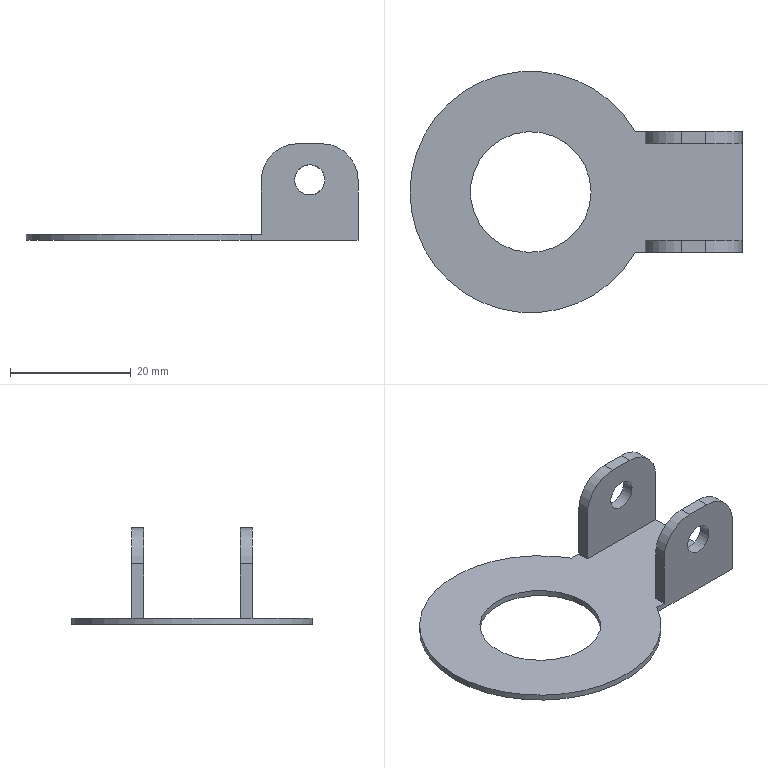Part | NX | features DATUM_CSYS 5, EXTRUDE 4, SKETCH 4, BLEND 1 | 1 solid | 19 faces | box 55 x 40 x 16 mm | volume 2079 mm3 | plane 11 | cylinder 8 | commonest cylinder face diameters 12 x4 5 x2 20 x1 40 x1
STEP:
#1=CARTESIAN_POINT('',(17.321,10.,0.));
#2=VERTEX_POINT('',#1);
#3=CARTESIAN_POINT('',(17.321,-10.,0.));
#4=VERTEX_POINT('',#3);
#5=CARTESIAN_POINT('',(0.,0.,0.));
#6=DIRECTION('',(0.,0.,1.));
#7=DIRECTION('',(1.,0.,0.));
#8=AXIS2_PLACEMENT_3D('',#5,#6,#7);
#9=CIRCLE('',#8,20.);
#10=EDGE_CURVE('',#2,#4,#9,.T.);
#11=ORIENTED_EDGE('',*,*,#10,.T.);
#12=CARTESIAN_POINT('',(17.321,-10.,1.));
#13=VERTEX_POINT('',#12);
#14=CARTESIAN_POINT('',(17.321,-10.,1.));
#15=DIRECTION('',(0.,0.,-1.));
#16=VECTOR('',#15,1000.);
#17=LINE('',#14,#16);
#18=EDGE_CURVE('',#4,#13,#17,.F.);
#19=ORIENTED_EDGE('',*,*,#18,.T.);
#20=CARTESIAN_POINT('',(17.321,10.,1.));
#21=VERTEX_POINT('',#20);
#22=CARTESIAN_POINT('',(0.,0.,1.));
#23=DIRECTION('',(0.,0.,1.));
#24=DIRECTION('',(1.,0.,0.));
#25=AXIS2_PLACEMENT_3D('',#22,#23,#24);
#26=CIRCLE('',#25,20.);
#27=EDGE_CURVE('',#21,#13,#26,.T.);
#28=ORIENTED_EDGE('',*,*,#27,.F.);
#29=CARTESIAN_POINT('',(17.321,10.,1.));
#30=DIRECTION('',(0.,0.,-1.));
#31=VECTOR('',#30,1000.);
#32=LINE('',#29,#31);
#33=EDGE_CURVE('',#21,#2,#32,.T.);
#34=ORIENTED_EDGE('',*,*,#33,.T.);
#35=EDGE_LOOP('',(#11,#19,#28,#34));
#36=FACE_BOUND('',#35,.T.);
#37=CARTESIAN_POINT('',(0.,0.,1.));
#38=DIRECTION('',(0.,0.,-1.));
#39=DIRECTION('',(-1.,0.,0.));
#40=AXIS2_PLACEMENT_3D('',#37,#38,#39);
#41=CYLINDRICAL_SURFACE('',#40,20.);
#42=ADVANCED_FACE('',(#36),#41,.T.);
#43=CARTESIAN_POINT('',(10.,0.,1.));
#44=VERTEX_POINT('',#43);
#45=CARTESIAN_POINT('',(0.,0.,1.));
#46=DIRECTION('',(0.,0.,1.));
#47=DIRECTION('',(1.,0.,0.));
#48=AXIS2_PLACEMENT_3D('',#45,#46,#47);
#49=CIRCLE('',#48,10.);
#50=EDGE_CURVE('',#44,#44,#49,.T.);
#51=ORIENTED_EDGE('',*,*,#50,.T.);
#52=EDGE_LOOP('',(#51));
#53=FACE_BOUND('',#52,.T.);
#54=CARTESIAN_POINT('',(10.,0.,0.));
#55=VERTEX_POINT('',#54);
#56=CARTESIAN_POINT('',(0.,0.,0.));
#57=DIRECTION('',(0.,0.,1.));
#58=DIRECTION('',(1.,0.,0.));
#59=AXIS2_PLACEMENT_3D('',#56,#57,#58);
#60=CIRCLE('',#59,10.);
#61=EDGE_CURVE('',#55,#55,#60,.T.);
#62=ORIENTED_EDGE('',*,*,#61,.F.);
#63=EDGE_LOOP('',(#62));
#64=FACE_BOUND('',#63,.T.);
#65=CARTESIAN_POINT('',(0.,0.,1.));
#66=DIRECTION('',(0.,0.,-1.));
#67=DIRECTION('',(-1.,0.,0.));
#68=AXIS2_PLACEMENT_3D('',#65,#66,#67);
#69=CYLINDRICAL_SURFACE('',#68,10.);
#70=ADVANCED_FACE('',(#53,#64),#69,.F.);
#71=CARTESIAN_POINT('',(19.,-8.,1.));
#72=VERTEX_POINT('',#71);
#73=CARTESIAN_POINT('',(19.,-10.,1.));
#74=VERTEX_POINT('',#73);
#75=CARTESIAN_POINT('',(19.,-8.,1.));
#76=DIRECTION('',(0.,-1.,0.));
#77=VECTOR('',#76,1000.);
#78=LINE('',#75,#77);
#79=EDGE_CURVE('',#72,#74,#78,.T.);
#80=ORIENTED_EDGE('',*,*,#79,.F.);
#81=CARTESIAN_POINT('',(35.,-8.,1.));
#82=VERTEX_POINT('',#81);
#83=CARTESIAN_POINT('',(35.,-8.,1.));
#84=DIRECTION('',(-1.,0.,0.));
#85=VECTOR('',#84,1000.);
#86=LINE('',#83,#85);
#87=EDGE_CURVE('',#82,#72,#86,.T.);
#88=ORIENTED_EDGE('',*,*,#87,.F.);
#89=CARTESIAN_POINT('',(35.,8.,1.));
#90=VERTEX_POINT('',#89);
#91=CARTESIAN_POINT('',(35.,-10.,1.));
#92=DIRECTION('',(0.,1.,0.));
#93=VECTOR('',#92,1000.);
#94=LINE('',#91,#93);
#95=EDGE_CURVE('',#82,#90,#94,.T.);
#96=ORIENTED_EDGE('',*,*,#95,.T.);
#97=CARTESIAN_POINT('',(19.,8.,1.));
#98=VERTEX_POINT('',#97);
#99=CARTESIAN_POINT('',(19.,8.,1.));
#100=DIRECTION('',(1.,0.,0.));
#101=VECTOR('',#100,1000.);
#102=LINE('',#99,#101);
#103=EDGE_CURVE('',#98,#90,#102,.T.);
#104=ORIENTED_EDGE('',*,*,#103,.F.);
#105=CARTESIAN_POINT('',(19.,10.,1.));
#106=VERTEX_POINT('',#105);
#107=CARTESIAN_POINT('',(19.,10.,1.));
#108=DIRECTION('',(0.,-1.,0.));
#109=VECTOR('',#108,1000.);
#110=LINE('',#107,#109);
#111=EDGE_CURVE('',#106,#98,#110,.T.);
#112=ORIENTED_EDGE('',*,*,#111,.F.);
#113=CARTESIAN_POINT('',(35.,10.,1.));
#114=DIRECTION('',(-1.,0.,0.));
#115=VECTOR('',#114,1000.);
#116=LINE('',#113,#115);
#117=EDGE_CURVE('',#106,#21,#116,.T.);
#118=ORIENTED_EDGE('',*,*,#117,.T.);
#119=ORIENTED_EDGE('',*,*,#27,.T.);
#120=CARTESIAN_POINT('',(15.,-10.,1.));
#121=DIRECTION('',(1.,0.,0.));
#122=VECTOR('',#121,1000.);
#123=LINE('',#120,#122);
#124=EDGE_CURVE('',#13,#74,#123,.T.);
#125=ORIENTED_EDGE('',*,*,#124,.T.);
#126=EDGE_LOOP('',(#80,#88,#96,#104,#112,#118,#119,#125));
#127=FACE_BOUND('',#126,.T.);
#128=ORIENTED_EDGE('',*,*,#50,.F.);
#129=EDGE_LOOP('',(#128));
#130=FACE_BOUND('',#129,.T.);
#131=CARTESIAN_POINT('',(0.,0.,1.));
#132=DIRECTION('',(0.,0.,1.));
#133=DIRECTION('',(1.,0.,0.));
#134=AXIS2_PLACEMENT_3D('',#131,#132,#133);
#135=PLANE('',#134);
#136=ADVANCED_FACE('',(#127,#130),#135,.T.);
#137=ORIENTED_EDGE('',*,*,#10,.F.);
#138=CARTESIAN_POINT('',(35.,10.,0.));
#139=VERTEX_POINT('',#138);
#140=CARTESIAN_POINT('',(35.,10.,0.));
#141=DIRECTION('',(-1.,0.,0.));
#142=VECTOR('',#141,1000.);
#143=LINE('',#140,#142);
#144=EDGE_CURVE('',#139,#2,#143,.T.);
#145=ORIENTED_EDGE('',*,*,#144,.F.);
#146=CARTESIAN_POINT('',(35.,-10.,0.));
#147=VERTEX_POINT('',#146);
#148=CARTESIAN_POINT('',(35.,-10.,0.));
#149=DIRECTION('',(0.,1.,0.));
#150=VECTOR('',#149,1000.);
#151=LINE('',#148,#150);
#152=EDGE_CURVE('',#147,#139,#151,.T.);
#153=ORIENTED_EDGE('',*,*,#152,.F.);
#154=CARTESIAN_POINT('',(15.,-10.,0.));
#155=DIRECTION('',(1.,0.,0.));
#156=VECTOR('',#155,1000.);
#157=LINE('',#154,#156);
#158=EDGE_CURVE('',#4,#147,#157,.T.);
#159=ORIENTED_EDGE('',*,*,#158,.F.);
#160=EDGE_LOOP('',(#137,#145,#153,#159));
#161=FACE_BOUND('',#160,.T.);
#162=ORIENTED_EDGE('',*,*,#61,.T.);
#163=EDGE_LOOP('',(#162));
#164=FACE_BOUND('',#163,.T.);
#165=CARTESIAN_POINT('',(0.,0.,0.));
#166=DIRECTION('',(0.,0.,1.));
#167=DIRECTION('',(1.,0.,0.));
#168=AXIS2_PLACEMENT_3D('',#165,#166,#167);
#169=PLANE('',#168);
#170=ADVANCED_FACE('',(#161,#164),#169,.F.);
#171=CARTESIAN_POINT('',(29.5,-10.,10.));
#172=VERTEX_POINT('',#171);
#173=CARTESIAN_POINT('',(27.,-10.,10.));
#174=DIRECTION('',(0.,-1.,0.));
#175=DIRECTION('',(1.,0.,0.));
#176=AXIS2_PLACEMENT_3D('',#173,#174,#175);
#177=CIRCLE('',#176,2.5);
#178=EDGE_CURVE('',#172,#172,#177,.T.);
#179=ORIENTED_EDGE('',*,*,#178,.F.);
#180=EDGE_LOOP('',(#179));
#181=FACE_BOUND('',#180,.T.);
#182=CARTESIAN_POINT('',(35.,-10.,10.));
#183=VERTEX_POINT('',#182);
#184=CARTESIAN_POINT('',(35.,-10.,0.));
#185=DIRECTION('',(0.,0.,1.));
#186=VECTOR('',#185,1000.);
#187=LINE('',#184,#186);
#188=EDGE_CURVE('',#147,#183,#187,.T.);
#189=ORIENTED_EDGE('',*,*,#188,.T.);
#190=CARTESIAN_POINT('',(29.,-10.,16.));
#191=VERTEX_POINT('',#190);
#192=CARTESIAN_POINT('',(29.,-10.,10.));
#193=DIRECTION('',(0.,-1.,0.));
#194=DIRECTION('',(1.,0.,0.));
#195=AXIS2_PLACEMENT_3D('',#192,#193,#194);
#196=CIRCLE('',#195,6.);
#197=EDGE_CURVE('',#183,#191,#196,.T.);
#198=ORIENTED_EDGE('',*,*,#197,.T.);
#199=CARTESIAN_POINT('',(25.,-10.,16.));
#200=VERTEX_POINT('',#199);
#201=CARTESIAN_POINT('',(19.,-10.,16.));
#202=DIRECTION('',(1.,0.,0.));
#203=VECTOR('',#202,1000.);
#204=LINE('',#201,#203);
#205=EDGE_CURVE('',#200,#191,#204,.T.);
#206=ORIENTED_EDGE('',*,*,#205,.F.);
#207=CARTESIAN_POINT('',(19.,-10.,10.));
#208=VERTEX_POINT('',#207);
#209=CARTESIAN_POINT('',(25.,-10.,10.));
#210=DIRECTION('',(0.,-1.,0.));
#211=DIRECTION('',(1.,0.,0.));
#212=AXIS2_PLACEMENT_3D('',#209,#210,#211);
#213=CIRCLE('',#212,6.);
#214=EDGE_CURVE('',#200,#208,#213,.T.);
#215=ORIENTED_EDGE('',*,*,#214,.T.);
#216=CARTESIAN_POINT('',(19.,-10.,16.));
#217=DIRECTION('',(0.,0.,-1.));
#218=VECTOR('',#217,1000.);
#219=LINE('',#216,#218);
#220=EDGE_CURVE('',#208,#74,#219,.T.);
#221=ORIENTED_EDGE('',*,*,#220,.T.);
#222=ORIENTED_EDGE('',*,*,#124,.F.);
#223=ORIENTED_EDGE('',*,*,#18,.F.);
#224=ORIENTED_EDGE('',*,*,#158,.T.);
#225=EDGE_LOOP('',(#189,#198,#206,#215,#221,#222,#223,#224));
#226=FACE_BOUND('',#225,.T.);
#227=CARTESIAN_POINT('',(15.,-10.,0.));
#228=DIRECTION('',(0.,-1.,0.));
#229=DIRECTION('',(1.,0.,0.));
#230=AXIS2_PLACEMENT_3D('',#227,#228,#229);
#231=PLANE('',#230);
#232=ADVANCED_FACE('',(#181,#226),#231,.T.);
#233=CARTESIAN_POINT('',(24.5,10.,10.));
#234=VERTEX_POINT('',#233);
#235=CARTESIAN_POINT('',(27.,10.,10.));
#236=DIRECTION('',(0.,1.,0.));
#237=DIRECTION('',(-1.,0.,0.));
#238=AXIS2_PLACEMENT_3D('',#235,#236,#237);
#239=CIRCLE('',#238,2.5);
#240=EDGE_CURVE('',#234,#234,#239,.T.);
#241=ORIENTED_EDGE('',*,*,#240,.F.);
#242=EDGE_LOOP('',(#241));
#243=FACE_BOUND('',#242,.T.);
#244=CARTESIAN_POINT('',(19.,10.,10.));
#245=VERTEX_POINT('',#244);
#246=CARTESIAN_POINT('',(19.,10.,16.));
#247=DIRECTION('',(0.,0.,-1.));
#248=VECTOR('',#247,1000.);
#249=LINE('',#246,#248);
#250=EDGE_CURVE('',#245,#106,#249,.T.);
#251=ORIENTED_EDGE('',*,*,#250,.F.);
#252=CARTESIAN_POINT('',(25.,10.,16.));
#253=VERTEX_POINT('',#252);
#254=CARTESIAN_POINT('',(25.,10.,10.));
#255=DIRECTION('',(0.,1.,0.));
#256=DIRECTION('',(-1.,0.,0.));
#257=AXIS2_PLACEMENT_3D('',#254,#255,#256);
#258=CIRCLE('',#257,6.);
#259=EDGE_CURVE('',#245,#253,#258,.T.);
#260=ORIENTED_EDGE('',*,*,#259,.T.);
#261=CARTESIAN_POINT('',(29.,10.,16.));
#262=VERTEX_POINT('',#261);
#263=CARTESIAN_POINT('',(35.,10.,16.));
#264=DIRECTION('',(-1.,0.,0.));
#265=VECTOR('',#264,1000.);
#266=LINE('',#263,#265);
#267=EDGE_CURVE('',#262,#253,#266,.T.);
#268=ORIENTED_EDGE('',*,*,#267,.F.);
#269=CARTESIAN_POINT('',(35.,10.,10.));
#270=VERTEX_POINT('',#269);
#271=CARTESIAN_POINT('',(29.,10.,10.));
#272=DIRECTION('',(0.,1.,0.));
#273=DIRECTION('',(-1.,0.,0.));
#274=AXIS2_PLACEMENT_3D('',#271,#272,#273);
#275=CIRCLE('',#274,6.);
#276=EDGE_CURVE('',#262,#270,#275,.T.);
#277=ORIENTED_EDGE('',*,*,#276,.T.);
#278=CARTESIAN_POINT('',(35.,10.,0.));
#279=DIRECTION('',(0.,0.,1.));
#280=VECTOR('',#279,1000.);
#281=LINE('',#278,#280);
#282=EDGE_CURVE('',#139,#270,#281,.T.);
#283=ORIENTED_EDGE('',*,*,#282,.F.);
#284=ORIENTED_EDGE('',*,*,#144,.T.);
#285=ORIENTED_EDGE('',*,*,#33,.F.);
#286=ORIENTED_EDGE('',*,*,#117,.F.);
#287=EDGE_LOOP('',(#251,#260,#268,#277,#283,#284,#285,#286));
#288=FACE_BOUND('',#287,.T.);
#289=CARTESIAN_POINT('',(35.,10.,0.));
#290=DIRECTION('',(0.,1.,0.));
#291=DIRECTION('',(-1.,0.,0.));
#292=AXIS2_PLACEMENT_3D('',#289,#290,#291);
#293=PLANE('',#292);
#294=ADVANCED_FACE('',(#243,#288),#293,.T.);
#295=ORIENTED_EDGE('',*,*,#282,.T.);
#296=CARTESIAN_POINT('',(35.,8.,10.));
#297=VERTEX_POINT('',#296);
#298=CARTESIAN_POINT('',(35.,-10.,10.));
#299=DIRECTION('',(0.,1.,0.));
#300=VECTOR('',#299,1000.);
#301=LINE('',#298,#300);
#302=EDGE_CURVE('',#270,#297,#301,.F.);
#303=ORIENTED_EDGE('',*,*,#302,.T.);
#304=CARTESIAN_POINT('',(35.,8.,16.));
#305=DIRECTION('',(0.,0.,-1.));
#306=VECTOR('',#305,1000.);
#307=LINE('',#304,#306);
#308=EDGE_CURVE('',#297,#90,#307,.T.);
#309=ORIENTED_EDGE('',*,*,#308,.T.);
#310=ORIENTED_EDGE('',*,*,#95,.F.);
#311=CARTESIAN_POINT('',(35.,-8.,10.));
#312=VERTEX_POINT('',#311);
#313=CARTESIAN_POINT('',(35.,-8.,16.));
#314=DIRECTION('',(0.,0.,-1.));
#315=VECTOR('',#314,1000.);
#316=LINE('',#313,#315);
#317=EDGE_CURVE('',#312,#82,#316,.T.);
#318=ORIENTED_EDGE('',*,*,#317,.F.);
#319=CARTESIAN_POINT('',(35.,-10.,10.));
#320=DIRECTION('',(0.,1.,0.));
#321=VECTOR('',#320,1000.);
#322=LINE('',#319,#321);
#323=EDGE_CURVE('',#312,#183,#322,.F.);
#324=ORIENTED_EDGE('',*,*,#323,.T.);
#325=ORIENTED_EDGE('',*,*,#188,.F.);
#326=ORIENTED_EDGE('',*,*,#152,.T.);
#327=EDGE_LOOP('',(#295,#303,#309,#310,#318,#324,#325,#326));
#328=FACE_BOUND('',#327,.T.);
#329=CARTESIAN_POINT('',(35.,-10.,0.));
#330=DIRECTION('',(1.,0.,0.));
#331=DIRECTION('',(0.,0.,-1.));
#332=AXIS2_PLACEMENT_3D('',#329,#330,#331);
#333=PLANE('',#332);
#334=ADVANCED_FACE('',(#328),#333,.T.);
#335=CARTESIAN_POINT('',(19.,8.,10.));
#336=VERTEX_POINT('',#335);
#337=CARTESIAN_POINT('',(19.,8.,16.));
#338=DIRECTION('',(0.,0.,-1.));
#339=VECTOR('',#338,1000.);
#340=LINE('',#337,#339);
#341=EDGE_CURVE('',#336,#98,#340,.T.);
#342=ORIENTED_EDGE('',*,*,#341,.F.);
#343=CARTESIAN_POINT('',(19.,10.,10.));
#344=DIRECTION('',(0.,-1.,0.));
#345=VECTOR('',#344,1000.);
#346=LINE('',#343,#345);
#347=EDGE_CURVE('',#336,#245,#346,.F.);
#348=ORIENTED_EDGE('',*,*,#347,.T.);
#349=ORIENTED_EDGE('',*,*,#250,.T.);
#350=ORIENTED_EDGE('',*,*,#111,.T.);
#351=EDGE_LOOP('',(#342,#348,#349,#350));
#352=FACE_BOUND('',#351,.T.);
#353=CARTESIAN_POINT('',(19.,10.,16.));
#354=DIRECTION('',(1.,0.,0.));
#355=DIRECTION('',(0.,0.,-1.));
#356=AXIS2_PLACEMENT_3D('',#353,#354,#355);
#357=PLANE('',#356);
#358=ADVANCED_FACE('',(#352),#357,.F.);
#359=CARTESIAN_POINT('',(27.,8.,12.5));
#360=VERTEX_POINT('',#359);
#361=CARTESIAN_POINT('',(27.,8.,10.));
#362=DIRECTION('',(0.,1.,0.));
#363=DIRECTION('',(0.,0.,1.));
#364=AXIS2_PLACEMENT_3D('',#361,#362,#363);
#365=CIRCLE('',#364,2.5);
#366=EDGE_CURVE('',#360,#360,#365,.T.);
#367=ORIENTED_EDGE('',*,*,#366,.T.);
#368=EDGE_LOOP('',(#367));
#369=FACE_BOUND('',#368,.T.);
#370=CARTESIAN_POINT('',(25.,8.,16.));
#371=VERTEX_POINT('',#370);
#372=CARTESIAN_POINT('',(29.,8.,16.));
#373=VERTEX_POINT('',#372);
#374=CARTESIAN_POINT('',(19.,8.,16.));
#375=DIRECTION('',(1.,0.,0.));
#376=VECTOR('',#375,1000.);
#377=LINE('',#374,#376);
#378=EDGE_CURVE('',#371,#373,#377,.T.);
#379=ORIENTED_EDGE('',*,*,#378,.F.);
#380=CARTESIAN_POINT('',(25.,8.,10.));
#381=DIRECTION('',(0.,1.,0.));
#382=DIRECTION('',(0.,0.,1.));
#383=AXIS2_PLACEMENT_3D('',#380,#381,#382);
#384=CIRCLE('',#383,6.);
#385=EDGE_CURVE('',#371,#336,#384,.F.);
#386=ORIENTED_EDGE('',*,*,#385,.T.);
#387=ORIENTED_EDGE('',*,*,#341,.T.);
#388=ORIENTED_EDGE('',*,*,#103,.T.);
#389=ORIENTED_EDGE('',*,*,#308,.F.);
#390=CARTESIAN_POINT('',(29.,8.,10.));
#391=DIRECTION('',(0.,1.,0.));
#392=DIRECTION('',(0.,0.,1.));
#393=AXIS2_PLACEMENT_3D('',#390,#391,#392);
#394=CIRCLE('',#393,6.);
#395=EDGE_CURVE('',#297,#373,#394,.F.);
#396=ORIENTED_EDGE('',*,*,#395,.T.);
#397=EDGE_LOOP('',(#379,#386,#387,#388,#389,#396));
#398=FACE_BOUND('',#397,.T.);
#399=CARTESIAN_POINT('',(19.,8.,16.));
#400=DIRECTION('',(0.,1.,0.));
#401=DIRECTION('',(0.,0.,1.));
#402=AXIS2_PLACEMENT_3D('',#399,#400,#401);
#403=PLANE('',#402);
#404=ADVANCED_FACE('',(#369,#398),#403,.F.);
#405=ORIENTED_EDGE('',*,*,#267,.T.);
#406=CARTESIAN_POINT('',(25.,8.,16.));
#407=DIRECTION('',(0.,-1.,0.));
#408=VECTOR('',#407,1000.);
#409=LINE('',#406,#408);
#410=EDGE_CURVE('',#253,#371,#409,.T.);
#411=ORIENTED_EDGE('',*,*,#410,.T.);
#412=ORIENTED_EDGE('',*,*,#378,.T.);
#413=CARTESIAN_POINT('',(29.,0.,16.));
#414=DIRECTION('',(0.,1.,0.));
#415=VECTOR('',#414,1000.);
#416=LINE('',#413,#415);
#417=EDGE_CURVE('',#373,#262,#416,.T.);
#418=ORIENTED_EDGE('',*,*,#417,.T.);
#419=EDGE_LOOP('',(#405,#411,#412,#418));
#420=FACE_BOUND('',#419,.T.);
#421=CARTESIAN_POINT('',(0.,0.,16.));
#422=DIRECTION('',(0.,0.,1.));
#423=DIRECTION('',(1.,0.,0.));
#424=AXIS2_PLACEMENT_3D('',#421,#422,#423);
#425=PLANE('',#424);
#426=ADVANCED_FACE('',(#420),#425,.T.);
#427=ORIENTED_EDGE('',*,*,#220,.F.);
#428=CARTESIAN_POINT('',(19.,-8.,10.));
#429=VERTEX_POINT('',#428);
#430=CARTESIAN_POINT('',(19.,-8.,10.));
#431=DIRECTION('',(0.,-1.,0.));
#432=VECTOR('',#431,1000.);
#433=LINE('',#430,#432);
#434=EDGE_CURVE('',#208,#429,#433,.F.);
#435=ORIENTED_EDGE('',*,*,#434,.T.);
#436=CARTESIAN_POINT('',(19.,-8.,16.));
#437=DIRECTION('',(0.,0.,-1.));
#438=VECTOR('',#437,1000.);
#439=LINE('',#436,#438);
#440=EDGE_CURVE('',#429,#72,#439,.T.);
#441=ORIENTED_EDGE('',*,*,#440,.T.);
#442=ORIENTED_EDGE('',*,*,#79,.T.);
#443=EDGE_LOOP('',(#427,#435,#441,#442));
#444=FACE_BOUND('',#443,.T.);
#445=CARTESIAN_POINT('',(19.,-8.,16.));
#446=DIRECTION('',(1.,0.,0.));
#447=DIRECTION('',(0.,0.,-1.));
#448=AXIS2_PLACEMENT_3D('',#445,#446,#447);
#449=PLANE('',#448);
#450=ADVANCED_FACE('',(#444),#449,.F.);
#451=CARTESIAN_POINT('',(29.5,-8.,10.));
#452=VERTEX_POINT('',#451);
#453=CARTESIAN_POINT('',(27.,-8.,10.));
#454=DIRECTION('',(0.,-1.,0.));
#455=DIRECTION('',(1.,0.,0.));
#456=AXIS2_PLACEMENT_3D('',#453,#454,#455);
#457=CIRCLE('',#456,2.5);
#458=EDGE_CURVE('',#452,#452,#457,.T.);
#459=ORIENTED_EDGE('',*,*,#458,.T.);
#460=EDGE_LOOP('',(#459));
#461=FACE_BOUND('',#460,.T.);
#462=CARTESIAN_POINT('',(29.,-8.,16.));
#463=VERTEX_POINT('',#462);
#464=CARTESIAN_POINT('',(25.,-8.,16.));
#465=VERTEX_POINT('',#464);
#466=CARTESIAN_POINT('',(35.,-8.,16.));
#467=DIRECTION('',(-1.,0.,0.));
#468=VECTOR('',#467,1000.);
#469=LINE('',#466,#468);
#470=EDGE_CURVE('',#463,#465,#469,.T.);
#471=ORIENTED_EDGE('',*,*,#470,.F.);
#472=CARTESIAN_POINT('',(29.,-8.,10.));
#473=DIRECTION('',(0.,-1.,0.));
#474=DIRECTION('',(1.,0.,0.));
#475=AXIS2_PLACEMENT_3D('',#472,#473,#474);
#476=CIRCLE('',#475,6.);
#477=EDGE_CURVE('',#463,#312,#476,.F.);
#478=ORIENTED_EDGE('',*,*,#477,.T.);
#479=ORIENTED_EDGE('',*,*,#317,.T.);
#480=ORIENTED_EDGE('',*,*,#87,.T.);
#481=ORIENTED_EDGE('',*,*,#440,.F.);
#482=CARTESIAN_POINT('',(25.,-8.,10.));
#483=DIRECTION('',(0.,-1.,0.));
#484=DIRECTION('',(1.,0.,0.));
#485=AXIS2_PLACEMENT_3D('',#482,#483,#484);
#486=CIRCLE('',#485,6.);
#487=EDGE_CURVE('',#429,#465,#486,.F.);
#488=ORIENTED_EDGE('',*,*,#487,.T.);
#489=EDGE_LOOP('',(#471,#478,#479,#480,#481,#488));
#490=FACE_BOUND('',#489,.T.);
#491=CARTESIAN_POINT('',(35.,-8.,16.));
#492=DIRECTION('',(0.,-1.,0.));
#493=DIRECTION('',(1.,0.,0.));
#494=AXIS2_PLACEMENT_3D('',#491,#492,#493);
#495=PLANE('',#494);
#496=ADVANCED_FACE('',(#461,#490),#495,.F.);
#497=ORIENTED_EDGE('',*,*,#205,.T.);
#498=CARTESIAN_POINT('',(29.,0.,16.));
#499=DIRECTION('',(0.,1.,0.));
#500=VECTOR('',#499,1000.);
#501=LINE('',#498,#500);
#502=EDGE_CURVE('',#191,#463,#501,.T.);
#503=ORIENTED_EDGE('',*,*,#502,.T.);
#504=ORIENTED_EDGE('',*,*,#470,.T.);
#505=CARTESIAN_POINT('',(25.,-10.,16.));
#506=DIRECTION('',(0.,-1.,0.));
#507=VECTOR('',#506,1000.);
#508=LINE('',#505,#507);
#509=EDGE_CURVE('',#465,#200,#508,.T.);
#510=ORIENTED_EDGE('',*,*,#509,.T.);
#511=EDGE_LOOP('',(#497,#503,#504,#510));
#512=FACE_BOUND('',#511,.T.);
#513=CARTESIAN_POINT('',(0.,0.,16.));
#514=DIRECTION('',(0.,0.,1.));
#515=DIRECTION('',(1.,0.,0.));
#516=AXIS2_PLACEMENT_3D('',#513,#514,#515);
#517=PLANE('',#516);
#518=ADVANCED_FACE('',(#512),#517,.T.);
#519=ORIENTED_EDGE('',*,*,#259,.F.);
#520=ORIENTED_EDGE('',*,*,#347,.F.);
#521=ORIENTED_EDGE('',*,*,#385,.F.);
#522=ORIENTED_EDGE('',*,*,#410,.F.);
#523=EDGE_LOOP('',(#519,#520,#521,#522));
#524=FACE_BOUND('',#523,.T.);
#525=CARTESIAN_POINT('',(25.,0.,10.));
#526=DIRECTION('',(0.,1.,0.));
#527=DIRECTION('',(0.,0.,1.));
#528=AXIS2_PLACEMENT_3D('',#525,#526,#527);
#529=CYLINDRICAL_SURFACE('',#528,6.);
#530=ADVANCED_FACE('',(#524),#529,.T.);
#531=ORIENTED_EDGE('',*,*,#395,.F.);
#532=ORIENTED_EDGE('',*,*,#302,.F.);
#533=ORIENTED_EDGE('',*,*,#276,.F.);
#534=ORIENTED_EDGE('',*,*,#417,.F.);
#535=EDGE_LOOP('',(#531,#532,#533,#534));
#536=FACE_BOUND('',#535,.T.);
#537=CARTESIAN_POINT('',(29.,0.,10.));
#538=DIRECTION('',(0.,1.,0.));
#539=DIRECTION('',(0.,0.,1.));
#540=AXIS2_PLACEMENT_3D('',#537,#538,#539);
#541=CYLINDRICAL_SURFACE('',#540,6.);
#542=ADVANCED_FACE('',(#536),#541,.T.);
#543=ORIENTED_EDGE('',*,*,#197,.F.);
#544=ORIENTED_EDGE('',*,*,#323,.F.);
#545=ORIENTED_EDGE('',*,*,#477,.F.);
#546=ORIENTED_EDGE('',*,*,#502,.F.);
#547=EDGE_LOOP('',(#543,#544,#545,#546));
#548=FACE_BOUND('',#547,.T.);
#549=CARTESIAN_POINT('',(29.,0.,10.));
#550=DIRECTION('',(0.,1.,0.));
#551=DIRECTION('',(0.,0.,1.));
#552=AXIS2_PLACEMENT_3D('',#549,#550,#551);
#553=CYLINDRICAL_SURFACE('',#552,6.);
#554=ADVANCED_FACE('',(#548),#553,.T.);
#555=ORIENTED_EDGE('',*,*,#487,.F.);
#556=ORIENTED_EDGE('',*,*,#434,.F.);
#557=ORIENTED_EDGE('',*,*,#214,.F.);
#558=ORIENTED_EDGE('',*,*,#509,.F.);
#559=EDGE_LOOP('',(#555,#556,#557,#558));
#560=FACE_BOUND('',#559,.T.);
#561=CARTESIAN_POINT('',(25.,0.,10.));
#562=DIRECTION('',(0.,1.,0.));
#563=DIRECTION('',(0.,0.,1.));
#564=AXIS2_PLACEMENT_3D('',#561,#562,#563);
#565=CYLINDRICAL_SURFACE('',#564,6.);
#566=ADVANCED_FACE('',(#560),#565,.T.);
#567=ORIENTED_EDGE('',*,*,#178,.T.);
#568=EDGE_LOOP('',(#567));
#569=FACE_BOUND('',#568,.T.);
#570=ORIENTED_EDGE('',*,*,#458,.F.);
#571=EDGE_LOOP('',(#570));
#572=FACE_BOUND('',#571,.T.);
#573=CARTESIAN_POINT('',(27.,47.,10.));
#574=DIRECTION('',(0.,-1.,0.));
#575=DIRECTION('',(0.,0.,-1.));
#576=AXIS2_PLACEMENT_3D('',#573,#574,#575);
#577=CYLINDRICAL_SURFACE('',#576,2.5);
#578=ADVANCED_FACE('',(#569,#572),#577,.F.);
#579=ORIENTED_EDGE('',*,*,#240,.T.);
#580=EDGE_LOOP('',(#579));
#581=FACE_BOUND('',#580,.T.);
#582=ORIENTED_EDGE('',*,*,#366,.F.);
#583=EDGE_LOOP('',(#582));
#584=FACE_BOUND('',#583,.T.);
#585=CARTESIAN_POINT('',(27.,47.,10.));
#586=DIRECTION('',(0.,-1.,0.));
#587=DIRECTION('',(0.,0.,-1.));
#588=AXIS2_PLACEMENT_3D('',#585,#586,#587);
#589=CYLINDRICAL_SURFACE('',#588,2.5);
#590=ADVANCED_FACE('',(#581,#584),#589,.F.);
#591=CLOSED_SHELL('',(#42,#70,#136,#170,#232,#294,#334,#358,#404,#426,#450,#496,#518,#530,#542,#554,#566,#578,#590));
#592=MANIFOLD_SOLID_BREP('',#591);
#593=(LENGTH_UNIT()NAMED_UNIT(*)SI_UNIT(.MILLI.,.METRE.));
#594=UNCERTAINTY_MEASURE_WITH_UNIT(LENGTH_MEASURE(0.00001),#593,'','');
#595=(NAMED_UNIT(*)PLANE_ANGLE_UNIT()SI_UNIT($,.RADIAN.));
#596=(NAMED_UNIT(*)SI_UNIT($,.STERADIAN.)SOLID_ANGLE_UNIT());
#597=(GEOMETRIC_REPRESENTATION_CONTEXT(3)GLOBAL_UNCERTAINTY_ASSIGNED_CONTEXT((#594))GLOBAL_UNIT_ASSIGNED_CONTEXT((#593,#595,#596))REPRESENTATION_CONTEXT('',''));
#598=ADVANCED_BREP_SHAPE_REPRESENTATION('',(#592),#597);